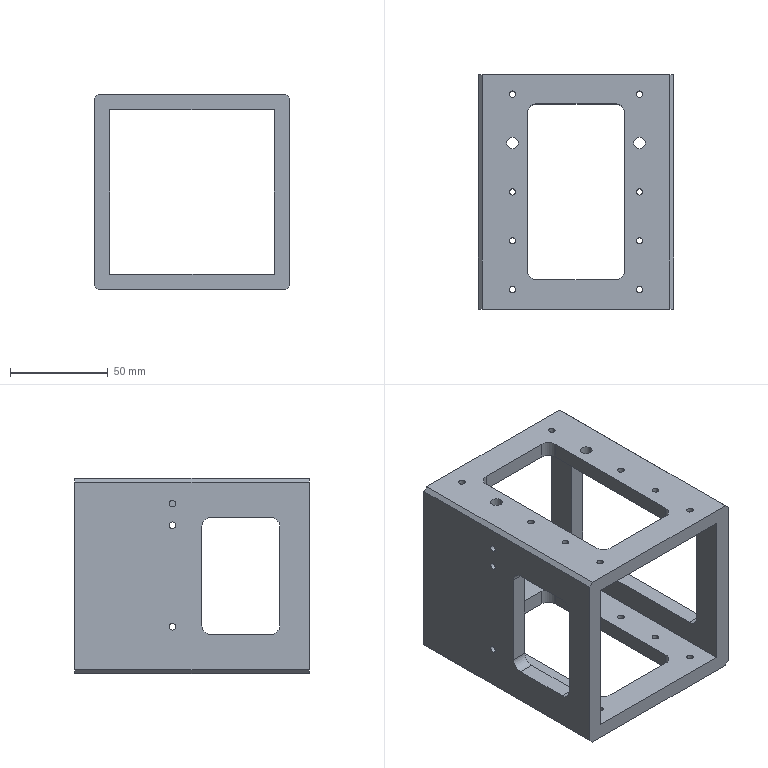Part | SolidWorks | features ICE 5, HoleWzd 4, MirrorPattern 2, 3DProfileFeature 1, Chamfer 1, Cut 1, Extrusion 1 | 1 solid | 92 faces | box 100 x 120 x 100 mm | volume 216402 mm3 | cylinder 62 | plane 30 | commonest cylinder face diameters 3.3 x38 10 x16 6 x8